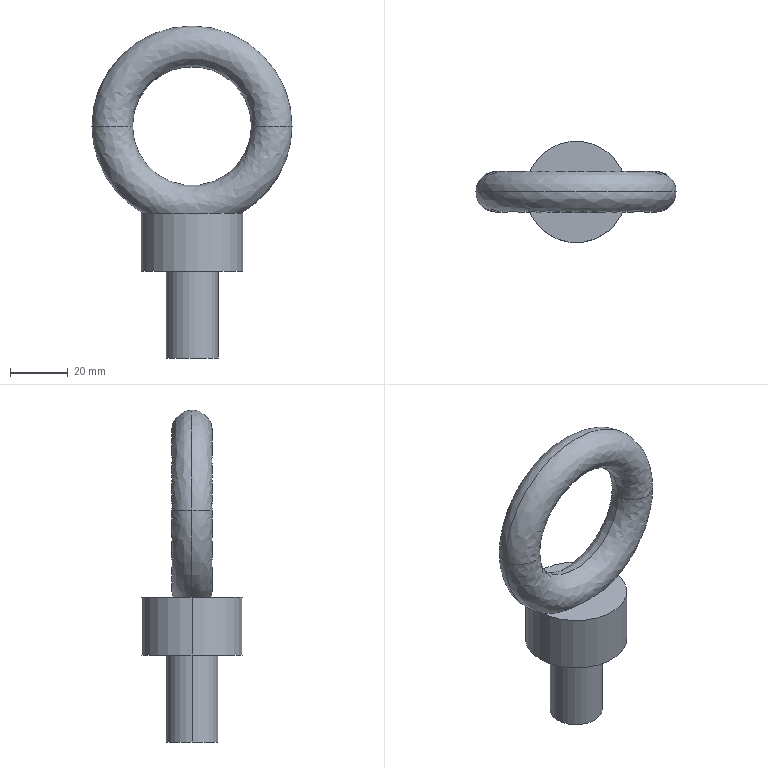Part | SolidWorks | features BaseBody 1 | 1 solid | 11 faces | box 69 x 35 x 114.5 mm | volume 52594 mm3 | spline 4 | cylinder 4 | plane 3 | commonest cylinder face diameters 18 x2 35 x2
STEP:
#1=CARTESIAN_POINT('',(917.446,-3900.973,2164.971));
#2=VERTEX_POINT('',#1);
#3=CARTESIAN_POINT('',(876.446,-3900.973,2164.971));
#4=VERTEX_POINT('',#3);
#5=CARTESIAN_POINT('',(896.946,-3900.973,2164.971));
#6=DIRECTION('',(0.,1.,0.));
#7=DIRECTION('',(-1.,0.,0.));
#8=AXIS2_PLACEMENT_3D('',#5,#6,#7);
#9=CIRCLE('',#8,20.5);
#10=EDGE_CURVE('',#2,#4,#9,.T.);
#11=ORIENTED_EDGE('',*,*,#10,.F.);
#12=CARTESIAN_POINT('',(931.446,-3900.973,2164.971));
#13=VERTEX_POINT('',#12);
#14=CARTESIAN_POINT('',(924.446,-3900.973,2164.971));
#15=DIRECTION('',(0.,0.,-1.));
#16=DIRECTION('',(1.,0.,0.));
#17=AXIS2_PLACEMENT_3D('',#14,#15,#16);
#18=CIRCLE('',#17,7.);
#19=EDGE_CURVE('',#2,#13,#18,.T.);
#20=ORIENTED_EDGE('',*,*,#19,.T.);
#21=CARTESIAN_POINT('',(913.982,-3900.973,2134.971));
#22=VERTEX_POINT('',#21);
#23=CARTESIAN_POINT('',(896.946,-3900.973,2164.971));
#24=DIRECTION('',(0.,1.,0.));
#25=DIRECTION('',(-1.,0.,0.));
#26=AXIS2_PLACEMENT_3D('',#23,#24,#25);
#27=CIRCLE('',#26,34.5);
#28=EDGE_CURVE('',#13,#22,#27,.T.);
#29=ORIENTED_EDGE('',*,*,#28,.T.);
#30=CARTESIAN_POINT('',(879.909,-3900.973,2134.971));
#31=VERTEX_POINT('',#30);
#32=CARTESIAN_POINT('',(913.982,-3900.973,2134.971));
#33=CARTESIAN_POINT('',(913.982,-3900.552,2134.971));
#34=CARTESIAN_POINT('',(913.906,-3900.145,2134.971));
#35=CARTESIAN_POINT('',(913.62,-3899.355,2134.971));
#36=CARTESIAN_POINT('',(913.416,-3898.992,2134.971));
#37=CARTESIAN_POINT('',(912.919,-3898.318,2134.971));
#38=CARTESIAN_POINT('',(912.633,-3898.018,2134.971));
#39=CARTESIAN_POINT('',(912.011,-3897.472,2134.971));
#40=CARTESIAN_POINT('',(911.671,-3897.225,2134.971));
#41=CARTESIAN_POINT('',(910.619,-3896.564,2134.971));
#42=CARTESIAN_POINT('',(909.869,-3896.222,2134.971));
#43=CARTESIAN_POINT('',(908.7,-3895.798,2134.971));
#44=CARTESIAN_POINT('',(908.303,-3895.673,2134.971));
#45=CARTESIAN_POINT('',(907.51,-3895.45,2134.971));
#46=CARTESIAN_POINT('',(907.111,-3895.351,2134.971));
#47=CARTESIAN_POINT('',(905.911,-3895.088,2134.971));
#48=CARTESIAN_POINT('',(905.105,-3894.954,2134.971));
#49=CARTESIAN_POINT('',(903.484,-3894.74,2134.971));
#50=CARTESIAN_POINT('',(902.67,-3894.662,2134.971));
#51=CARTESIAN_POINT('',(900.218,-3894.481,2134.971));
#52=CARTESIAN_POINT('',(898.572,-3894.434,2134.971));
#53=CARTESIAN_POINT('',(896.107,-3894.435,2134.971));
#54=CARTESIAN_POINT('',(895.285,-3894.448,2134.971));
#55=CARTESIAN_POINT('',(893.643,-3894.502,2134.971));
#56=CARTESIAN_POINT('',(892.821,-3894.543,2134.971));
#57=CARTESIAN_POINT('',(891.182,-3894.665,2134.971));
#58=CARTESIAN_POINT('',(890.366,-3894.745,2134.971));
#59=CARTESIAN_POINT('',(888.74,-3894.961,2134.971));
#60=CARTESIAN_POINT('',(887.93,-3895.097,2134.971));
#61=CARTESIAN_POINT('',(886.323,-3895.454,2134.971));
#62=CARTESIAN_POINT('',(885.529,-3895.674,2134.971));
#63=CARTESIAN_POINT('',(884.373,-3896.096,2134.971));
#64=CARTESIAN_POINT('',(883.994,-3896.253,2134.971));
#65=CARTESIAN_POINT('',(883.249,-3896.608,2134.971));
#66=CARTESIAN_POINT('',(882.885,-3896.805,2134.971));
#67=CARTESIAN_POINT('',(882.192,-3897.244,2134.971));
#68=CARTESIAN_POINT('',(881.86,-3897.487,2134.971));
#69=CARTESIAN_POINT('',(881.241,-3898.035,2134.971));
#70=CARTESIAN_POINT('',(880.957,-3898.337,2134.971));
#71=CARTESIAN_POINT('',(880.471,-3899.,2134.971));
#72=CARTESIAN_POINT('',(880.266,-3899.368,2134.971));
#73=CARTESIAN_POINT('',(879.986,-3900.141,2134.971));
#74=CARTESIAN_POINT('',(879.909,-3900.556,2134.971));
#75=CARTESIAN_POINT('',(879.909,-3900.973,2134.971));
#76=B_SPLINE_CURVE_WITH_KNOTS('',3,(#32,#33,#34,#35,#36,#37,#38,#39,#40,#41,#42,#43,#44,#45,#46,#47,#48,#49,#50,#51,#52,#53,#54,#55,#56,#57,#58,#59,#60,#61,#62,#63,#64,#65,#66,#67,#68,#69,#70,#71,#72,#73,#74,#75),.UNSPECIFIED.,.F.,.F.,(4,2,2,2,2,2,2,2,2,2,2,2,2,2,2,2,2,2,2,2,2,4),(0.01968,0.02091,0.02214,0.02338,0.02461,0.02708,0.02831,0.02954,0.03201,0.03448,0.03941,0.04188,0.04434,0.04681,0.04928,0.05174,0.05297,0.05421,0.05544,0.05667,0.05791,0.05914),.UNSPECIFIED.);
#77=EDGE_CURVE('',#22,#31,#76,.T.);
#78=ORIENTED_EDGE('',*,*,#77,.T.);
#79=CARTESIAN_POINT('',(862.446,-3900.973,2164.971));
#80=VERTEX_POINT('',#79);
#81=CARTESIAN_POINT('',(896.946,-3900.973,2164.971));
#82=DIRECTION('',(0.,1.,0.));
#83=DIRECTION('',(-1.,0.,0.));
#84=AXIS2_PLACEMENT_3D('',#81,#82,#83);
#85=CIRCLE('',#84,34.5);
#86=EDGE_CURVE('',#31,#80,#85,.T.);
#87=ORIENTED_EDGE('',*,*,#86,.T.);
#88=CARTESIAN_POINT('',(869.446,-3900.973,2164.971));
#89=DIRECTION('',(0.,0.,1.));
#90=DIRECTION('',(-1.,0.,0.));
#91=AXIS2_PLACEMENT_3D('',#88,#89,#90);
#92=CIRCLE('',#91,7.);
#93=EDGE_CURVE('',#4,#80,#92,.T.);
#94=ORIENTED_EDGE('',*,*,#93,.F.);
#95=EDGE_LOOP('',(#11,#20,#29,#78,#87,#94));
#96=FACE_OUTER_BOUND('',#95,.T.);
#97=CARTESIAN_POINT('',(917.446,-3900.973,2164.971));
#98=CARTESIAN_POINT('',(917.446,-3900.973,2123.971));
#99=CARTESIAN_POINT('',(876.446,-3900.973,2123.971));
#100=CARTESIAN_POINT('',(876.446,-3900.973,2164.971));
#101=CARTESIAN_POINT('',(917.446,-3886.973,2164.971));
#102=CARTESIAN_POINT('',(917.446,-3886.973,2123.971));
#103=CARTESIAN_POINT('',(876.446,-3886.973,2123.971));
#104=CARTESIAN_POINT('',(876.446,-3886.973,2164.971));
#105=CARTESIAN_POINT('',(931.446,-3886.973,2164.971));
#106=CARTESIAN_POINT('',(931.446,-3886.973,2095.971));
#107=CARTESIAN_POINT('',(862.446,-3886.973,2095.971));
#108=CARTESIAN_POINT('',(862.446,-3886.973,2164.971));
#109=CARTESIAN_POINT('',(931.446,-3900.973,2164.971));
#110=CARTESIAN_POINT('',(931.446,-3900.973,2095.971));
#111=CARTESIAN_POINT('',(862.446,-3900.973,2095.971));
#112=CARTESIAN_POINT('',(862.446,-3900.973,2164.971));
#113=(BOUNDED_SURFACE()B_SPLINE_SURFACE(3,3,((#97,#98,#99,#100),(#101,#102,#103,#104),(#105,#106,#107,#108),(#109,#110,#111,#112)),.UNSPECIFIED.,.F.,.F.,.F.)B_SPLINE_SURFACE_WITH_KNOTS((4,4),(4,4),(0.,1.),(0.,1.),.UNSPECIFIED.)GEOMETRIC_REPRESENTATION_ITEM()RATIONAL_B_SPLINE_SURFACE(((1.,0.3333,0.3333,1.),(0.3333,0.1111,0.1111,0.3333),(0.3333,0.1111,0.1111,0.3333),(1.,0.3333,0.3333,1.)))REPRESENTATION_ITEM('')SURFACE());
#114=ADVANCED_FACE('',(#96),#113,.T.);
#115=ORIENTED_EDGE('',*,*,#28,.F.);
#116=CARTESIAN_POINT('',(924.446,-3900.973,2164.971));
#117=DIRECTION('',(0.,0.,-1.));
#118=DIRECTION('',(1.,0.,0.));
#119=AXIS2_PLACEMENT_3D('',#116,#117,#118);
#120=CIRCLE('',#119,7.);
#121=EDGE_CURVE('',#13,#2,#120,.T.);
#122=ORIENTED_EDGE('',*,*,#121,.T.);
#123=ORIENTED_EDGE('',*,*,#10,.T.);
#124=CARTESIAN_POINT('',(869.446,-3900.973,2164.971));
#125=DIRECTION('',(0.,0.,1.));
#126=DIRECTION('',(-1.,0.,0.));
#127=AXIS2_PLACEMENT_3D('',#124,#125,#126);
#128=CIRCLE('',#127,7.);
#129=EDGE_CURVE('',#80,#4,#128,.T.);
#130=ORIENTED_EDGE('',*,*,#129,.F.);
#131=ORIENTED_EDGE('',*,*,#86,.F.);
#132=CARTESIAN_POINT('',(879.909,-3900.973,2134.971));
#133=CARTESIAN_POINT('',(879.909,-3901.391,2134.971));
#134=CARTESIAN_POINT('',(879.984,-3901.797,2134.971));
#135=CARTESIAN_POINT('',(880.267,-3902.582,2134.971));
#136=CARTESIAN_POINT('',(880.469,-3902.944,2134.971));
#137=CARTESIAN_POINT('',(880.961,-3903.616,2134.971));
#138=CARTESIAN_POINT('',(881.244,-3903.914,2134.971));
#139=CARTESIAN_POINT('',(881.861,-3904.459,2134.971));
#140=CARTESIAN_POINT('',(882.198,-3904.706,2134.971));
#141=CARTESIAN_POINT('',(883.242,-3905.366,2134.971));
#142=CARTESIAN_POINT('',(883.987,-3905.708,2134.971));
#143=CARTESIAN_POINT('',(885.147,-3906.133,2134.971));
#144=CARTESIAN_POINT('',(885.541,-3906.259,2134.971));
#145=CARTESIAN_POINT('',(886.33,-3906.483,2134.971));
#146=CARTESIAN_POINT('',(886.726,-3906.582,2134.971));
#147=CARTESIAN_POINT('',(887.919,-3906.847,2134.971));
#148=CARTESIAN_POINT('',(888.72,-3906.982,2134.971));
#149=CARTESIAN_POINT('',(890.331,-3907.197,2134.971));
#150=CARTESIAN_POINT('',(891.14,-3907.277,2134.971));
#151=CARTESIAN_POINT('',(893.576,-3907.46,2134.971));
#152=CARTESIAN_POINT('',(895.213,-3907.509,2134.971));
#153=CARTESIAN_POINT('',(897.052,-3907.512,2134.971));
#154=CARTESIAN_POINT('',(897.26,-3907.511,2134.971));
#155=CARTESIAN_POINT('',(897.673,-3907.508,2134.971));
#156=CARTESIAN_POINT('',(897.88,-3907.506,2134.971));
#157=CARTESIAN_POINT('',(898.499,-3907.497,2134.971));
#158=CARTESIAN_POINT('',(898.912,-3907.488,2134.971));
#159=CARTESIAN_POINT('',(900.148,-3907.449,2134.971));
#160=CARTESIAN_POINT('',(900.972,-3907.408,2134.971));
#161=CARTESIAN_POINT('',(902.616,-3907.29,2134.971));
#162=CARTESIAN_POINT('',(903.436,-3907.211,2134.971));
#163=CARTESIAN_POINT('',(905.072,-3906.998,2134.971));
#164=CARTESIAN_POINT('',(905.89,-3906.863,2134.971));
#165=CARTESIAN_POINT('',(907.51,-3906.508,2134.971));
#166=CARTESIAN_POINT('',(908.309,-3906.289,2134.971));
#167=CARTESIAN_POINT('',(909.871,-3905.723,2134.971));
#168=CARTESIAN_POINT('',(910.621,-3905.381,2134.971));
#169=CARTESIAN_POINT('',(911.664,-3904.726,2134.971));
#170=CARTESIAN_POINT('',(911.999,-3904.484,2134.971));
#171=CARTESIAN_POINT('',(912.629,-3903.933,2134.971));
#172=CARTESIAN_POINT('',(912.917,-3903.631,2134.971));
#173=CARTESIAN_POINT('',(913.289,-3903.127,2134.971));
#174=CARTESIAN_POINT('',(913.403,-3902.95,2134.971));
#175=CARTESIAN_POINT('',(913.603,-3902.585,2134.971));
#176=CARTESIAN_POINT('',(913.69,-3902.397,2134.971));
#177=CARTESIAN_POINT('',(913.903,-3901.814,2134.971));
#178=CARTESIAN_POINT('',(913.982,-3901.395,2134.971));
#179=CARTESIAN_POINT('',(913.982,-3900.973,2134.971));
#180=B_SPLINE_CURVE_WITH_KNOTS('',3,(#132,#133,#134,#135,#136,#137,#138,#139,#140,#141,#142,#143,#144,#145,#146,#147,#148,#149,#150,#151,#152,#153,#154,#155,#156,#157,#158,#159,#160,#161,#162,#163,#164,#165,#166,#167,#168,#169,#170,#171,#172,#173,#174,#175,#176,#177,#178,#179),.UNSPECIFIED.,.F.,.F.,(4,2,2,2,2,2,2,2,2,2,2,2,2,2,2,2,2,2,2,2,2,2,2,4),(0.05914,0.06038,0.06161,0.06285,0.06409,0.06656,0.06779,0.06903,0.0715,0.07397,0.07892,0.07954,0.08015,0.08139,0.08386,0.08633,0.08881,0.09128,0.09375,0.09499,0.09622,0.09684,0.09746,0.09869),.UNSPECIFIED.);
#181=EDGE_CURVE('',#31,#22,#180,.T.);
#182=ORIENTED_EDGE('',*,*,#181,.T.);
#183=EDGE_LOOP('',(#115,#122,#123,#130,#131,#182));
#184=FACE_OUTER_BOUND('',#183,.T.);
#185=CARTESIAN_POINT('',(931.446,-3900.973,2164.971));
#186=CARTESIAN_POINT('',(931.446,-3900.973,2095.971));
#187=CARTESIAN_POINT('',(862.446,-3900.973,2095.971));
#188=CARTESIAN_POINT('',(862.446,-3900.973,2164.971));
#189=CARTESIAN_POINT('',(931.446,-3914.973,2164.971));
#190=CARTESIAN_POINT('',(931.446,-3914.973,2095.971));
#191=CARTESIAN_POINT('',(862.446,-3914.973,2095.971));
#192=CARTESIAN_POINT('',(862.446,-3914.973,2164.971));
#193=CARTESIAN_POINT('',(917.446,-3914.973,2164.971));
#194=CARTESIAN_POINT('',(917.446,-3914.973,2123.971));
#195=CARTESIAN_POINT('',(876.446,-3914.973,2123.971));
#196=CARTESIAN_POINT('',(876.446,-3914.973,2164.971));
#197=CARTESIAN_POINT('',(917.446,-3900.973,2164.971));
#198=CARTESIAN_POINT('',(917.446,-3900.973,2123.971));
#199=CARTESIAN_POINT('',(876.446,-3900.973,2123.971));
#200=CARTESIAN_POINT('',(876.446,-3900.973,2164.971));
#201=(BOUNDED_SURFACE()B_SPLINE_SURFACE(3,3,((#185,#186,#187,#188),(#189,#190,#191,#192),(#193,#194,#195,#196),(#197,#198,#199,#200)),.UNSPECIFIED.,.F.,.F.,.F.)B_SPLINE_SURFACE_WITH_KNOTS((4,4),(4,4),(0.,1.),(0.,1.),.UNSPECIFIED.)GEOMETRIC_REPRESENTATION_ITEM()RATIONAL_B_SPLINE_SURFACE(((1.,0.3333,0.3333,1.),(0.3333,0.1111,0.1111,0.3333),(0.3333,0.1111,0.1111,0.3333),(1.,0.3333,0.3333,1.)))REPRESENTATION_ITEM('')SURFACE());
#202=ADVANCED_FACE('',(#184),#201,.T.);
#203=ORIENTED_EDGE('',*,*,#121,.F.);
#204=CARTESIAN_POINT('',(896.946,-3900.973,2164.971));
#205=DIRECTION('',(0.,1.,0.));
#206=DIRECTION('',(-1.,0.,0.));
#207=AXIS2_PLACEMENT_3D('',#204,#205,#206);
#208=CIRCLE('',#207,34.5);
#209=EDGE_CURVE('',#80,#13,#208,.T.);
#210=ORIENTED_EDGE('',*,*,#209,.F.);
#211=ORIENTED_EDGE('',*,*,#129,.T.);
#212=CARTESIAN_POINT('',(896.946,-3900.973,2164.971));
#213=DIRECTION('',(0.,1.,0.));
#214=DIRECTION('',(-1.,0.,0.));
#215=AXIS2_PLACEMENT_3D('',#212,#213,#214);
#216=CIRCLE('',#215,20.5);
#217=EDGE_CURVE('',#4,#2,#216,.T.);
#218=ORIENTED_EDGE('',*,*,#217,.T.);
#219=EDGE_LOOP('',(#203,#210,#211,#218));
#220=FACE_OUTER_BOUND('',#219,.T.);
#221=CARTESIAN_POINT('',(862.446,-3900.973,2164.971));
#222=CARTESIAN_POINT('',(862.446,-3900.973,2233.971));
#223=CARTESIAN_POINT('',(931.446,-3900.973,2233.971));
#224=CARTESIAN_POINT('',(931.446,-3900.973,2164.971));
#225=CARTESIAN_POINT('',(862.446,-3914.973,2164.971));
#226=CARTESIAN_POINT('',(862.446,-3914.973,2233.971));
#227=CARTESIAN_POINT('',(931.446,-3914.973,2233.971));
#228=CARTESIAN_POINT('',(931.446,-3914.973,2164.971));
#229=CARTESIAN_POINT('',(876.446,-3914.973,2164.971));
#230=CARTESIAN_POINT('',(876.446,-3914.973,2205.971));
#231=CARTESIAN_POINT('',(917.446,-3914.973,2205.971));
#232=CARTESIAN_POINT('',(917.446,-3914.973,2164.971));
#233=CARTESIAN_POINT('',(876.446,-3900.973,2164.971));
#234=CARTESIAN_POINT('',(876.446,-3900.973,2205.971));
#235=CARTESIAN_POINT('',(917.446,-3900.973,2205.971));
#236=CARTESIAN_POINT('',(917.446,-3900.973,2164.971));
#237=(BOUNDED_SURFACE()B_SPLINE_SURFACE(3,3,((#221,#222,#223,#224),(#225,#226,#227,#228),(#229,#230,#231,#232),(#233,#234,#235,#236)),.UNSPECIFIED.,.F.,.F.,.F.)B_SPLINE_SURFACE_WITH_KNOTS((4,4),(4,4),(0.,1.),(0.,1.),.UNSPECIFIED.)GEOMETRIC_REPRESENTATION_ITEM()RATIONAL_B_SPLINE_SURFACE(((1.,0.3333,0.3333,1.),(0.3333,0.1111,0.1111,0.3333),(0.3333,0.1111,0.1111,0.3333),(1.,0.3333,0.3333,1.)))REPRESENTATION_ITEM('')SURFACE());
#238=ADVANCED_FACE('',(#220),#237,.T.);
#239=CARTESIAN_POINT('',(914.492,-3900.973,2114.971));
#240=VERTEX_POINT('',#239);
#241=CARTESIAN_POINT('',(879.492,-3900.973,2114.971));
#242=VERTEX_POINT('',#241);
#243=CARTESIAN_POINT('',(896.992,-3900.973,2114.971));
#244=DIRECTION('',(0.,0.,1.));
#245=DIRECTION('',(1.,0.,0.));
#246=AXIS2_PLACEMENT_3D('',#243,#244,#245);
#247=CIRCLE('',#246,17.5);
#248=EDGE_CURVE('',#240,#242,#247,.T.);
#249=ORIENTED_EDGE('',*,*,#248,.T.);
#250=CARTESIAN_POINT('',(879.492,-3900.973,2134.971));
#251=VERTEX_POINT('',#250);
#252=CARTESIAN_POINT('',(879.492,-3900.973,2124.971));
#253=DIRECTION('',(0.,0.,1.));
#254=VECTOR('',#253,1000.);
#255=LINE('',#252,#254);
#256=EDGE_CURVE('',#242,#251,#255,.T.);
#257=ORIENTED_EDGE('',*,*,#256,.T.);
#258=CARTESIAN_POINT('',(914.492,-3900.973,2134.971));
#259=VERTEX_POINT('',#258);
#260=CARTESIAN_POINT('',(896.992,-3900.973,2134.971));
#261=DIRECTION('',(0.,0.,1.));
#262=DIRECTION('',(1.,0.,0.));
#263=AXIS2_PLACEMENT_3D('',#260,#261,#262);
#264=CIRCLE('',#263,17.5);
#265=EDGE_CURVE('',#259,#251,#264,.T.);
#266=ORIENTED_EDGE('',*,*,#265,.F.);
#267=CARTESIAN_POINT('',(914.492,-3900.973,2124.971));
#268=DIRECTION('',(0.,0.,1.));
#269=VECTOR('',#268,1000.);
#270=LINE('',#267,#269);
#271=EDGE_CURVE('',#240,#259,#270,.T.);
#272=ORIENTED_EDGE('',*,*,#271,.F.);
#273=EDGE_LOOP('',(#249,#257,#266,#272));
#274=FACE_OUTER_BOUND('',#273,.T.);
#275=CARTESIAN_POINT('',(896.992,-3900.973,2124.971));
#276=DIRECTION('',(0.,0.,1.));
#277=DIRECTION('',(1.,0.,0.));
#278=AXIS2_PLACEMENT_3D('',#275,#276,#277);
#279=CYLINDRICAL_SURFACE('',#278,17.5);
#280=ADVANCED_FACE('',(#274),#279,.T.);
#281=CARTESIAN_POINT('',(905.992,-3900.973,2084.971));
#282=VERTEX_POINT('',#281);
#283=CARTESIAN_POINT('',(887.992,-3900.973,2084.971));
#284=VERTEX_POINT('',#283);
#285=CARTESIAN_POINT('',(896.992,-3900.973,2084.971));
#286=DIRECTION('',(0.,0.,1.));
#287=DIRECTION('',(1.,0.,0.));
#288=AXIS2_PLACEMENT_3D('',#285,#286,#287);
#289=CIRCLE('',#288,9.);
#290=EDGE_CURVE('',#282,#284,#289,.T.);
#291=ORIENTED_EDGE('',*,*,#290,.T.);
#292=CARTESIAN_POINT('',(887.992,-3900.973,2114.971));
#293=VERTEX_POINT('',#292);
#294=CARTESIAN_POINT('',(887.992,-3900.973,2099.971));
#295=DIRECTION('',(0.,0.,1.));
#296=VECTOR('',#295,1000.);
#297=LINE('',#294,#296);
#298=EDGE_CURVE('',#284,#293,#297,.T.);
#299=ORIENTED_EDGE('',*,*,#298,.T.);
#300=CARTESIAN_POINT('',(905.992,-3900.973,2114.971));
#301=VERTEX_POINT('',#300);
#302=CARTESIAN_POINT('',(896.992,-3900.973,2114.971));
#303=DIRECTION('',(0.,0.,1.));
#304=DIRECTION('',(1.,0.,0.));
#305=AXIS2_PLACEMENT_3D('',#302,#303,#304);
#306=CIRCLE('',#305,9.);
#307=EDGE_CURVE('',#301,#293,#306,.T.);
#308=ORIENTED_EDGE('',*,*,#307,.F.);
#309=CARTESIAN_POINT('',(905.992,-3900.973,2099.971));
#310=DIRECTION('',(0.,0.,1.));
#311=VECTOR('',#310,1000.);
#312=LINE('',#309,#311);
#313=EDGE_CURVE('',#282,#301,#312,.T.);
#314=ORIENTED_EDGE('',*,*,#313,.F.);
#315=EDGE_LOOP('',(#291,#299,#308,#314));
#316=FACE_OUTER_BOUND('',#315,.T.);
#317=CARTESIAN_POINT('',(896.992,-3900.973,2099.971));
#318=DIRECTION('',(0.,0.,1.));
#319=DIRECTION('',(1.,0.,0.));
#320=AXIS2_PLACEMENT_3D('',#317,#318,#319);
#321=CYLINDRICAL_SURFACE('',#320,9.);
#322=ADVANCED_FACE('',(#316),#321,.T.);
#323=ORIENTED_EDGE('',*,*,#19,.F.);
#324=ORIENTED_EDGE('',*,*,#217,.F.);
#325=ORIENTED_EDGE('',*,*,#93,.T.);
#326=ORIENTED_EDGE('',*,*,#209,.T.);
#327=EDGE_LOOP('',(#323,#324,#325,#326));
#328=FACE_OUTER_BOUND('',#327,.T.);
#329=CARTESIAN_POINT('',(876.446,-3900.973,2164.971));
#330=CARTESIAN_POINT('',(876.446,-3900.973,2205.971));
#331=CARTESIAN_POINT('',(917.446,-3900.973,2205.971));
#332=CARTESIAN_POINT('',(917.446,-3900.973,2164.971));
#333=CARTESIAN_POINT('',(876.446,-3886.973,2164.971));
#334=CARTESIAN_POINT('',(876.446,-3886.973,2205.971));
#335=CARTESIAN_POINT('',(917.446,-3886.973,2205.971));
#336=CARTESIAN_POINT('',(917.446,-3886.973,2164.971));
#337=CARTESIAN_POINT('',(862.446,-3886.973,2164.971));
#338=CARTESIAN_POINT('',(862.446,-3886.973,2233.971));
#339=CARTESIAN_POINT('',(931.446,-3886.973,2233.971));
#340=CARTESIAN_POINT('',(931.446,-3886.973,2164.971));
#341=CARTESIAN_POINT('',(862.446,-3900.973,2164.971));
#342=CARTESIAN_POINT('',(862.446,-3900.973,2233.971));
#343=CARTESIAN_POINT('',(931.446,-3900.973,2233.971));
#344=CARTESIAN_POINT('',(931.446,-3900.973,2164.971));
#345=(BOUNDED_SURFACE()B_SPLINE_SURFACE(3,3,((#329,#330,#331,#332),(#333,#334,#335,#336),(#337,#338,#339,#340),(#341,#342,#343,#344)),.UNSPECIFIED.,.F.,.F.,.F.)B_SPLINE_SURFACE_WITH_KNOTS((4,4),(4,4),(0.,1.),(0.,1.),.UNSPECIFIED.)GEOMETRIC_REPRESENTATION_ITEM()RATIONAL_B_SPLINE_SURFACE(((1.,0.3333,0.3333,1.),(0.3333,0.1111,0.1111,0.3333),(0.3333,0.1111,0.1111,0.3333),(1.,0.3333,0.3333,1.)))REPRESENTATION_ITEM('')SURFACE());
#346=ADVANCED_FACE('',(#328),#345,.T.);
#347=ORIENTED_EDGE('',*,*,#265,.T.);
#348=CARTESIAN_POINT('',(896.992,-3900.973,2134.971));
#349=DIRECTION('',(0.,0.,1.));
#350=DIRECTION('',(1.,0.,0.));
#351=AXIS2_PLACEMENT_3D('',#348,#349,#350);
#352=CIRCLE('',#351,17.5);
#353=EDGE_CURVE('',#251,#259,#352,.T.);
#354=ORIENTED_EDGE('',*,*,#353,.T.);
#355=EDGE_LOOP('',(#347,#354));
#356=FACE_OUTER_BOUND('',#355,.T.);
#357=ORIENTED_EDGE('',*,*,#77,.F.);
#358=ORIENTED_EDGE('',*,*,#181,.F.);
#359=EDGE_LOOP('',(#357,#358));
#360=FACE_BOUND('',#359,.T.);
#361=CARTESIAN_POINT('',(896.992,-3900.973,2134.971));
#362=DIRECTION('',(0.,0.,1.));
#363=DIRECTION('',(1.,0.,0.));
#364=AXIS2_PLACEMENT_3D('',#361,#362,#363);
#365=PLANE('',#364);
#366=ADVANCED_FACE('',(#356,#360),#365,.T.);
#367=ORIENTED_EDGE('',*,*,#256,.F.);
#368=CARTESIAN_POINT('',(896.992,-3900.973,2114.971));
#369=DIRECTION('',(0.,0.,1.));
#370=DIRECTION('',(1.,0.,0.));
#371=AXIS2_PLACEMENT_3D('',#368,#369,#370);
#372=CIRCLE('',#371,17.5);
#373=EDGE_CURVE('',#242,#240,#372,.T.);
#374=ORIENTED_EDGE('',*,*,#373,.T.);
#375=ORIENTED_EDGE('',*,*,#271,.T.);
#376=ORIENTED_EDGE('',*,*,#353,.F.);
#377=EDGE_LOOP('',(#367,#374,#375,#376));
#378=FACE_OUTER_BOUND('',#377,.T.);
#379=CARTESIAN_POINT('',(896.992,-3900.973,2124.971));
#380=DIRECTION('',(0.,0.,1.));
#381=DIRECTION('',(1.,0.,0.));
#382=AXIS2_PLACEMENT_3D('',#379,#380,#381);
#383=CYLINDRICAL_SURFACE('',#382,17.5);
#384=ADVANCED_FACE('',(#378),#383,.T.);
#385=ORIENTED_EDGE('',*,*,#248,.F.);
#386=ORIENTED_EDGE('',*,*,#373,.F.);
#387=EDGE_LOOP('',(#385,#386));
#388=FACE_OUTER_BOUND('',#387,.T.);
#389=ORIENTED_EDGE('',*,*,#307,.T.);
#390=CARTESIAN_POINT('',(896.992,-3900.973,2114.971));
#391=DIRECTION('',(0.,0.,1.));
#392=DIRECTION('',(1.,0.,0.));
#393=AXIS2_PLACEMENT_3D('',#390,#391,#392);
#394=CIRCLE('',#393,9.);
#395=EDGE_CURVE('',#293,#301,#394,.T.);
#396=ORIENTED_EDGE('',*,*,#395,.T.);
#397=EDGE_LOOP('',(#389,#396));
#398=FACE_BOUND('',#397,.T.);
#399=CARTESIAN_POINT('',(896.992,-3900.973,2114.971));
#400=DIRECTION('',(0.,0.,-1.));
#401=DIRECTION('',(-1.,0.,0.));
#402=AXIS2_PLACEMENT_3D('',#399,#400,#401);
#403=PLANE('',#402);
#404=ADVANCED_FACE('',(#388,#398),#403,.T.);
#405=ORIENTED_EDGE('',*,*,#298,.F.);
#406=CARTESIAN_POINT('',(896.992,-3900.973,2084.971));
#407=DIRECTION('',(0.,0.,1.));
#408=DIRECTION('',(1.,0.,0.));
#409=AXIS2_PLACEMENT_3D('',#406,#407,#408);
#410=CIRCLE('',#409,9.);
#411=EDGE_CURVE('',#284,#282,#410,.T.);
#412=ORIENTED_EDGE('',*,*,#411,.T.);
#413=ORIENTED_EDGE('',*,*,#313,.T.);
#414=ORIENTED_EDGE('',*,*,#395,.F.);
#415=EDGE_LOOP('',(#405,#412,#413,#414));
#416=FACE_OUTER_BOUND('',#415,.T.);
#417=CARTESIAN_POINT('',(896.992,-3900.973,2099.971));
#418=DIRECTION('',(0.,0.,1.));
#419=DIRECTION('',(1.,0.,0.));
#420=AXIS2_PLACEMENT_3D('',#417,#418,#419);
#421=CYLINDRICAL_SURFACE('',#420,9.);
#422=ADVANCED_FACE('',(#416),#421,.T.);
#423=ORIENTED_EDGE('',*,*,#290,.F.);
#424=ORIENTED_EDGE('',*,*,#411,.F.);
#425=EDGE_LOOP('',(#423,#424));
#426=FACE_OUTER_BOUND('',#425,.T.);
#427=CARTESIAN_POINT('',(896.992,-3900.973,2084.971));
#428=DIRECTION('',(0.,0.,-1.));
#429=DIRECTION('',(-1.,0.,0.));
#430=AXIS2_PLACEMENT_3D('',#427,#428,#429);
#431=PLANE('',#430);
#432=ADVANCED_FACE('',(#426),#431,.T.);
#433=CLOSED_SHELL('',(#114,#202,#238,#280,#322,#346,#366,#384,#404,#422,#432));
#434=MANIFOLD_SOLID_BREP('',#433);
#435=CARTESIAN_POINT('',(0.,0.,0.));
#436=DIRECTION('',(0.,0.,1.));
#437=DIRECTION('',(1.,0.,0.));
#438=AXIS2_PLACEMENT_3D('',#435,#436,#437);
#439=(LENGTH_UNIT()NAMED_UNIT(*)SI_UNIT(.MILLI.,.METRE.));
#440=UNCERTAINTY_MEASURE_WITH_UNIT(LENGTH_MEASURE(0.00001),#439,'','');
#441=(NAMED_UNIT(*)PLANE_ANGLE_UNIT()SI_UNIT($,.RADIAN.));
#442=(NAMED_UNIT(*)SI_UNIT($,.STERADIAN.)SOLID_ANGLE_UNIT());
#443=(GEOMETRIC_REPRESENTATION_CONTEXT(3)GLOBAL_UNCERTAINTY_ASSIGNED_CONTEXT((#440))GLOBAL_UNIT_ASSIGNED_CONTEXT((#439,#441,#442))REPRESENTATION_CONTEXT('',''));
#444=ADVANCED_BREP_SHAPE_REPRESENTATION('',(#434,#438),#443);